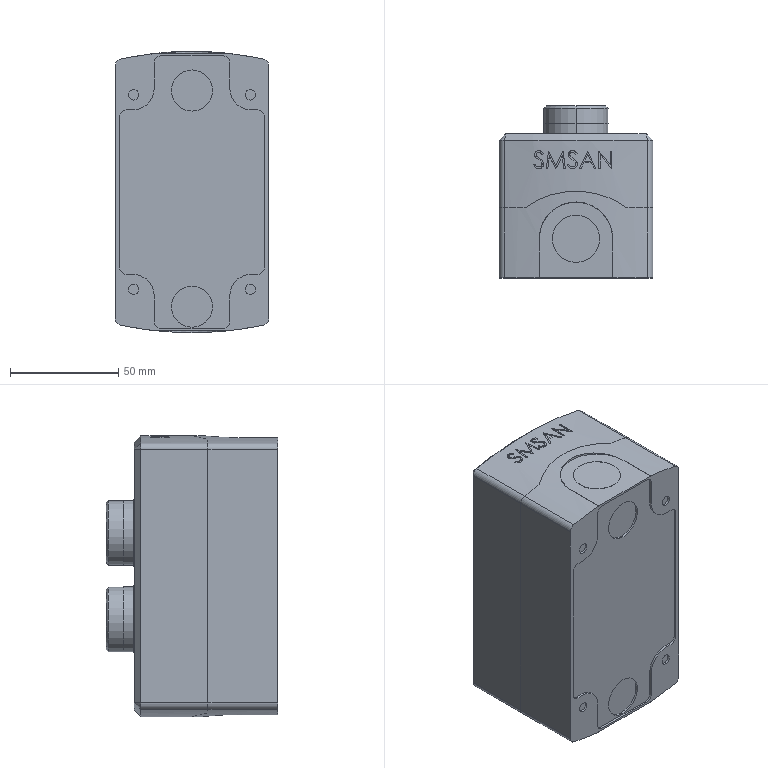Part | STEP file | 2 reset flat push button[GOB-2A10M-GW]_10M | 4 solids | 470 faces | box 71 x 79.5 x 130.1 mm | volume 149787 mm3 | plane 231 | cylinder 114 | spline 111 | cone 14 | commonest cylinder face diameters 6 x16 26.5 x10 2 x8 4.8 x8 8 x8 9 x8